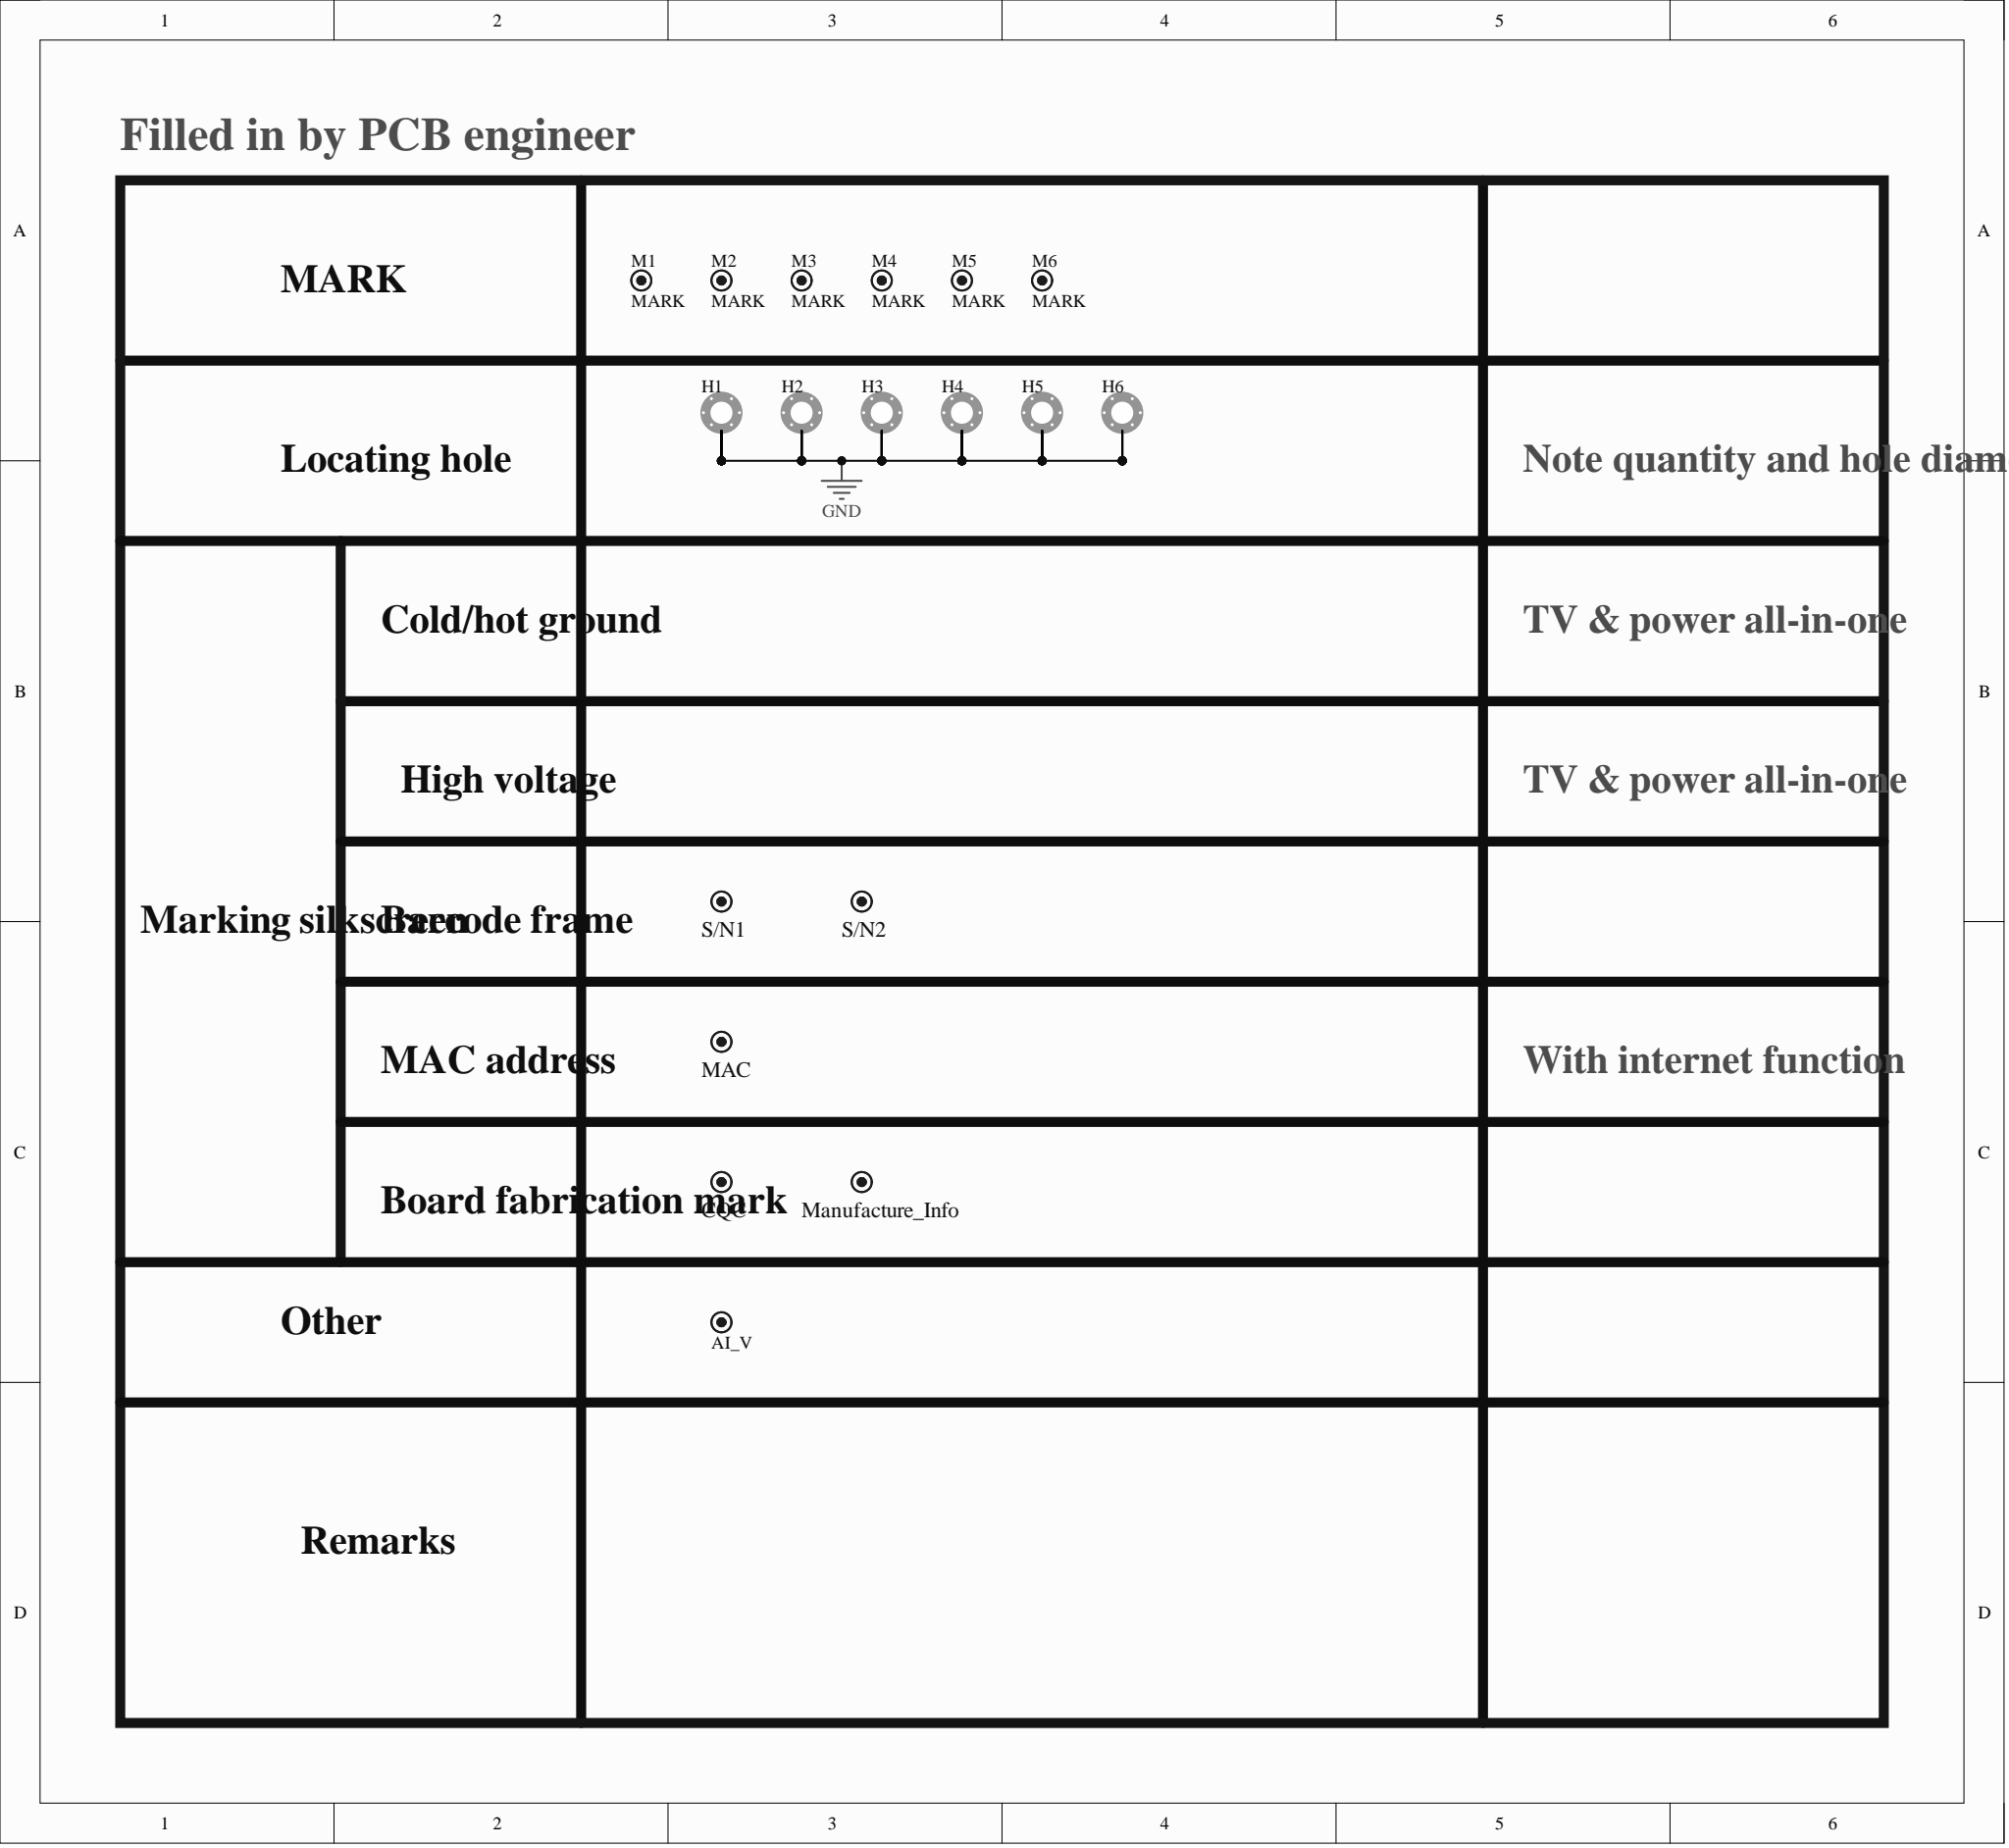Circuit board | Altium Designer | 1029 parts | 642 nets | one sheet of the schematic
Parts on this sheet (reference | value | footprint):
AI_V | AI_GRIPPER_V | AI_GRIPPER_V
CQC | CQC | CQC
M1 | MARK | MARK
M2 | MARK | MARK
M3 | MARK | MARK
M4 | MARK | MARK
M5 | MARK | MARK
M6 | MARK | MARK
MAC | MAC | Barcode
Manufacture_Info | Manufacture_Info | Manufacture_Info
S/N1 | Barcode | Barcode
S/N2 | Barcode | Barcode
Nets of these parts (net: part-pin ...):